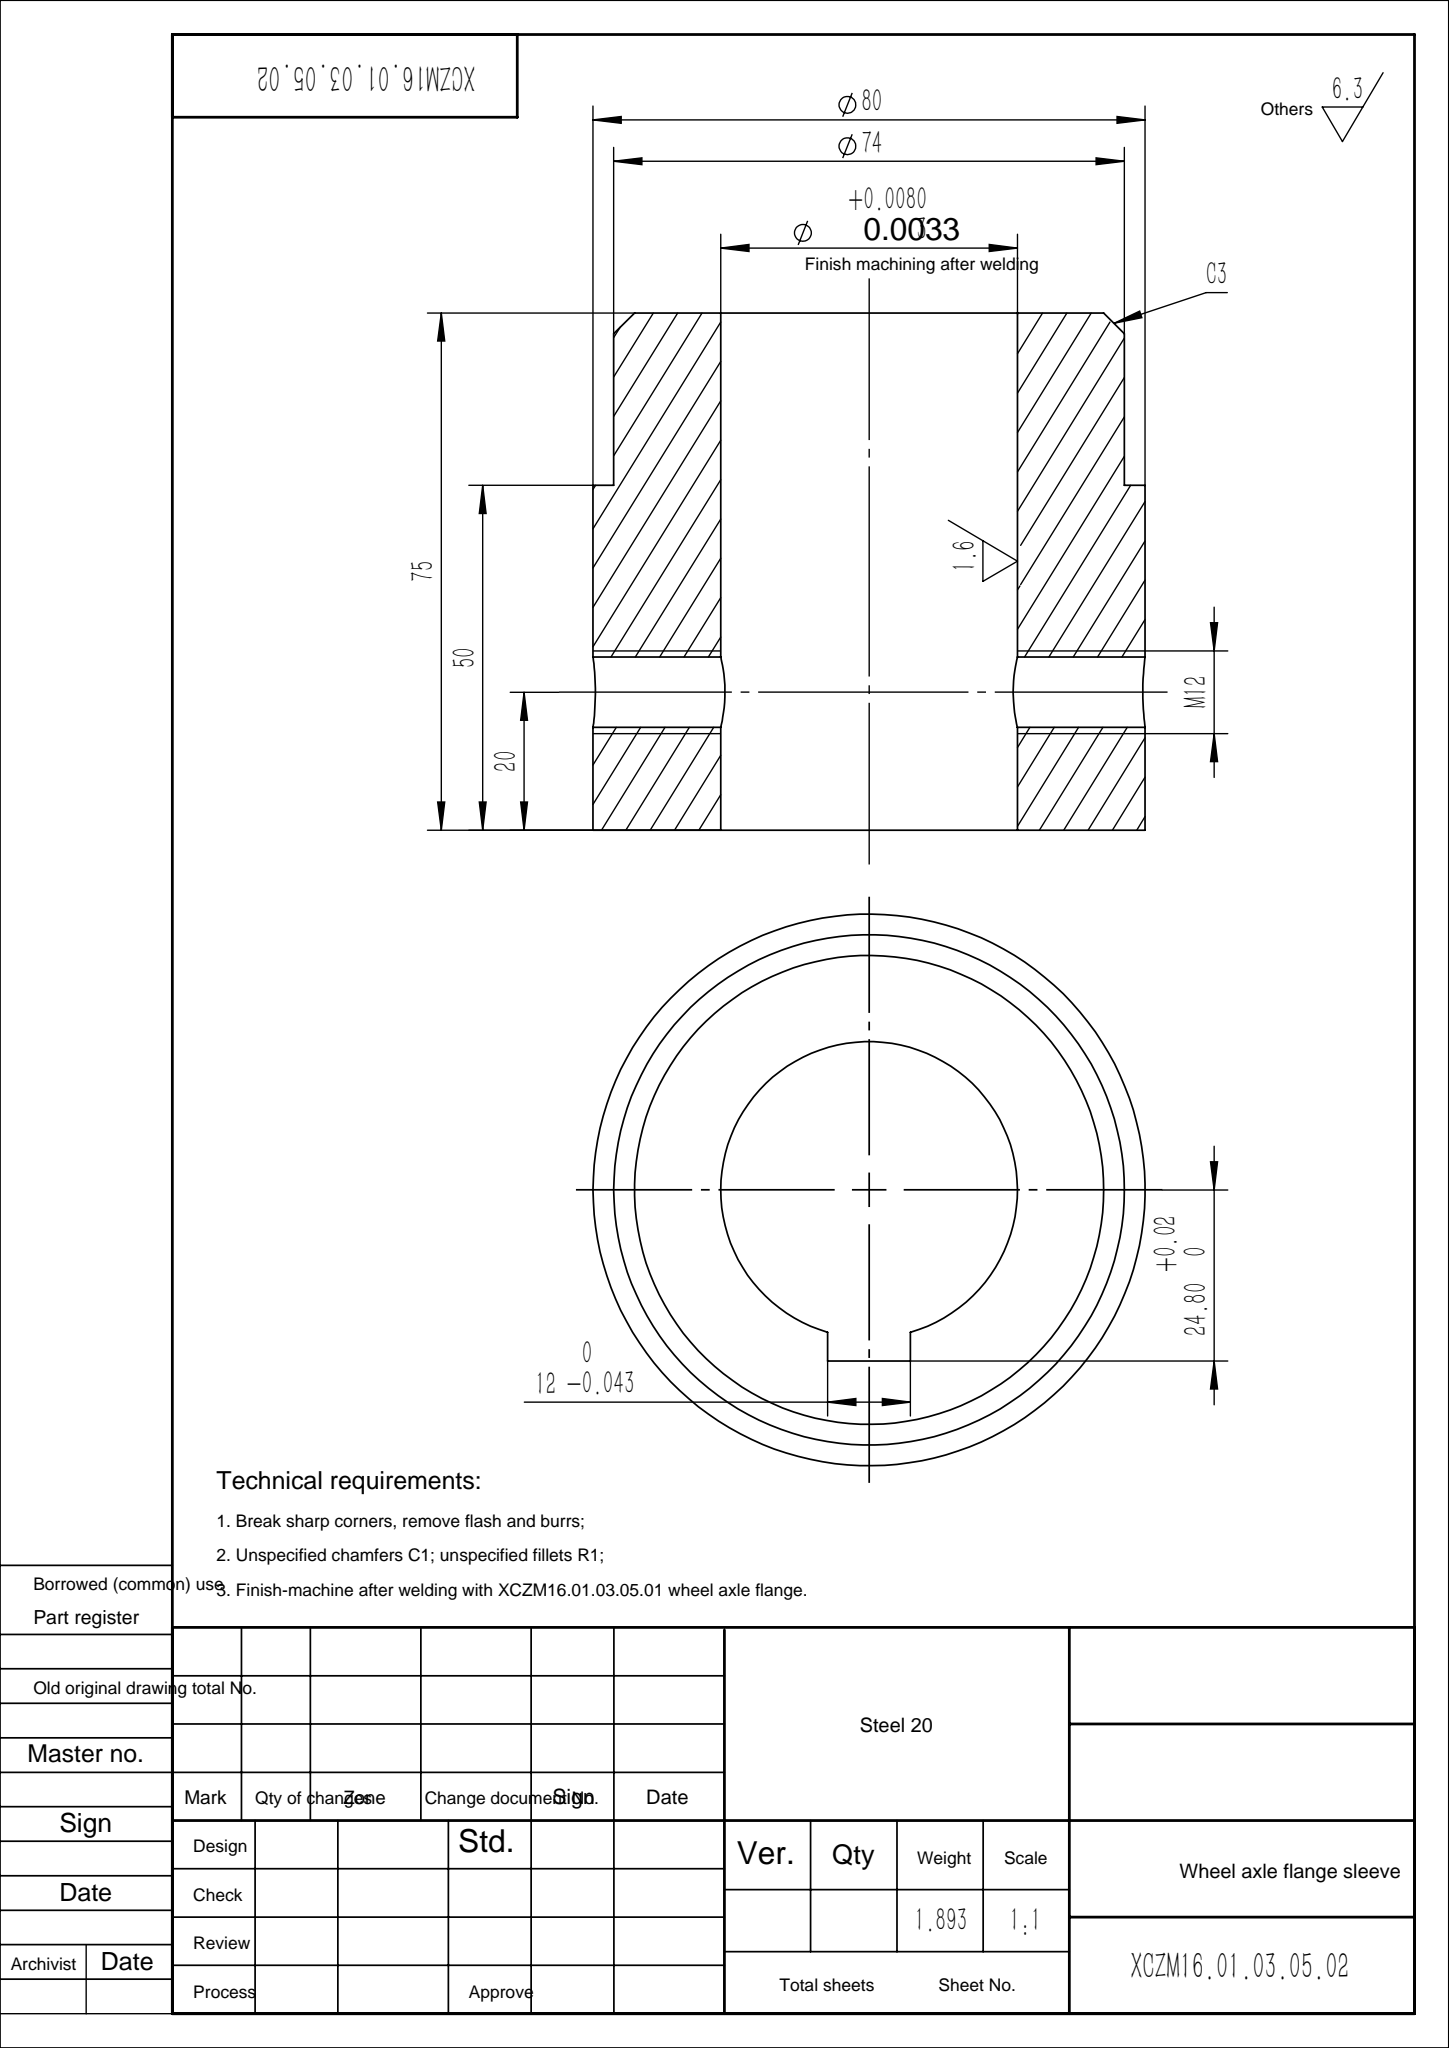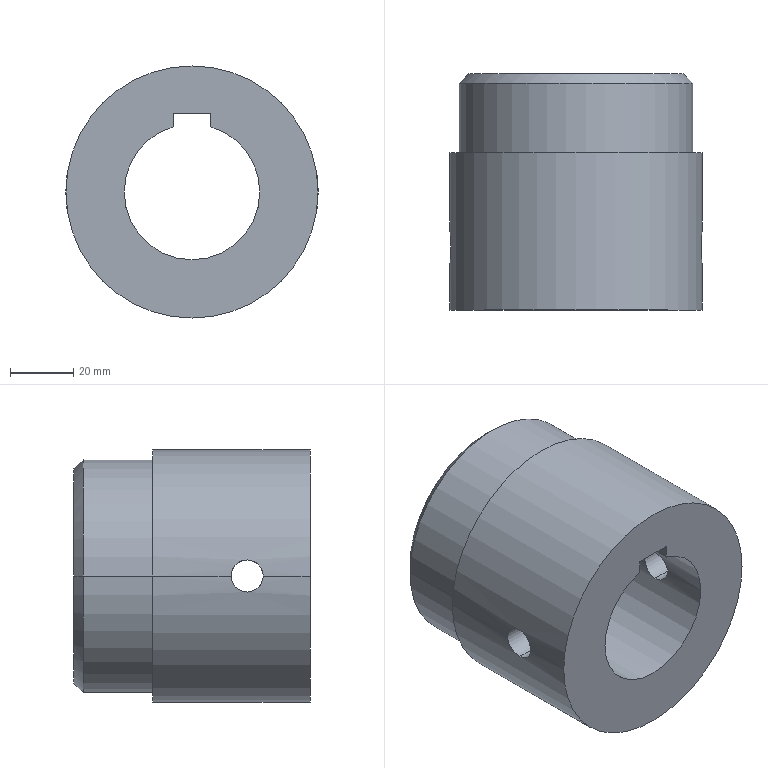Part | SolidWorks | features Chamfer 1, HoleWzd 1, ICE 1, Revolution 1 | 1 solid | 19 faces | box 80 x 75 x 80 mm | volume 242656 mm3 | cylinder 11 | plane 6 | cone 2 | commonest cylinder face diameters 10.2 x4 43 x3 74 x2 80 x2